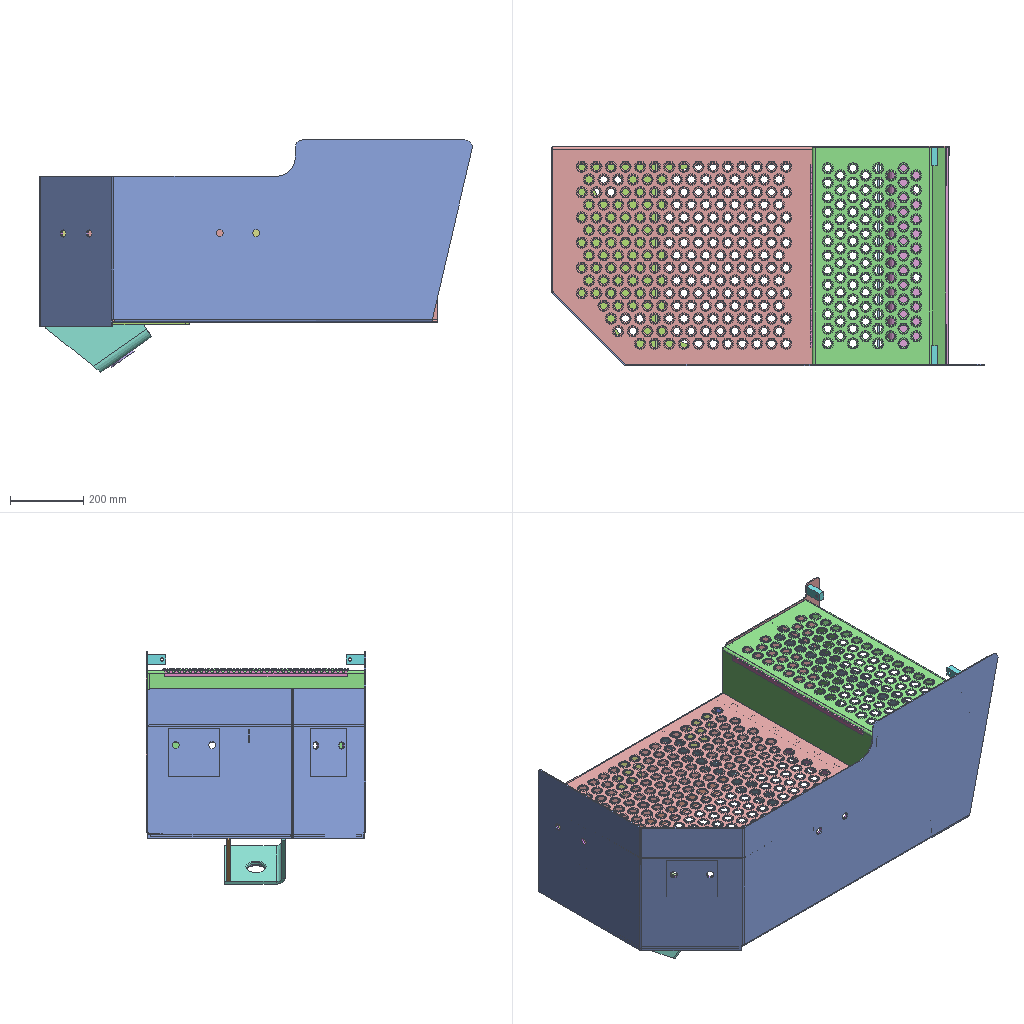Assembly | SolidWorks | 19 different items | 26 placed | box 1185 x 600 x 636 mm
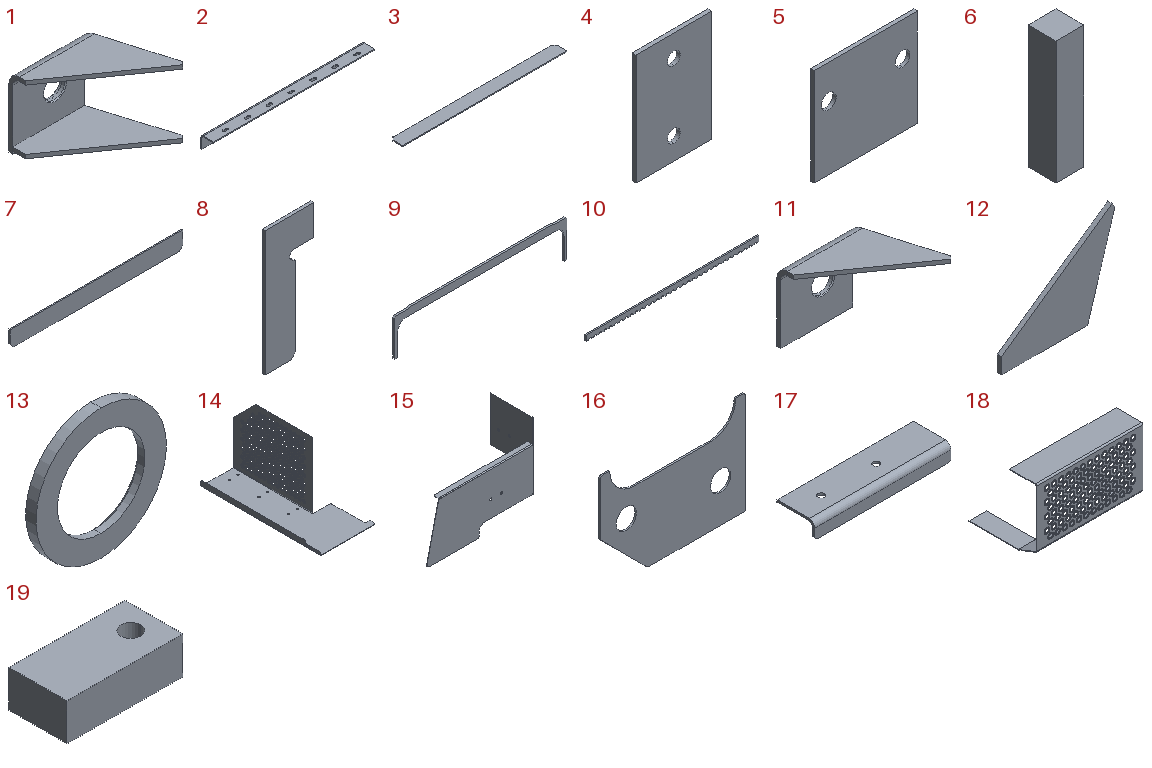Parts list (item | name | quantity | parent item | size | volume | features):
1 | (subassembly) | x1 | - | 224.289 x 199.117 x 166 mm | 593730 mm3 | features CosmeticWeldCutList 1
2 | - | x1 | - | 589 x 47 x 45 mm | 158032 mm3 | features FlatPattern 1, ICE 1, SMBaseFlange 1, SheetMetal 1
3 | - | x2 | - | 593.5 x 45 x 3.2 mm | 85144 mm3 | features Chamfer 1, FlatPattern 1, SMBaseFlange 1, SheetMetal 1
4 | - | x3 | - | 90 x 4.5 x 132 mm | 51870 mm3 | features FlatPattern 1, SMBaseFlange 1, SheetMetal 1
5 | - | x3 | - | 140 x 4.5 x 132 mm | 80333 mm3 | features FlatPattern 1, SMBaseFlange 1, SheetMetal 1
6 | - | x2 | - | 9 x 9 x 40 mm | 3240 mm3 | features FlatPattern 1, SMBaseFlange 1, SheetMetal 1
7 | - | x1 | - | 466 x 3.2 x 45 mm | 66784 mm3 | features FlatPattern 1, SMBaseFlange 1, SheetMetal 1
8 | - | x1 | - | 80 x 4.5 x 206 mm | 52392 mm3 | features FlatPattern 1, SMBaseFlange 1, SheetMetal 1
9 | - | x1 | - | 593.5 x 6 x 130 mm | 101926 mm3 | features FlatPattern 1, SMBaseFlange 1, SheetMetal 1
10 | - | x1 | - | 500 x 4.5 x 16 mm | 32268 mm3 | features FlatPattern 1, ICE 1, SMBaseFlange 1, SheetMetal 1
11 | - | x1 | in 1 | 224.289 x 193.117 x 166 mm | 401605 mm3 | features ICE 2, Chamfer 1, FlatPattern 1, SMBaseFlange 1, SheetMetal 1
12 | - | x1 | in 1 | 224.107 x 9 x 184.117 mm | 177492 mm3 | features FlatPattern 1, SMBaseFlange 1, SheetMetal 1
13 | - | x1 | in 1 | 76 x 6 x 76 mm | 14633 mm3 | features Chamfer 1, FlatPattern 1, SMBaseFlange 1, SheetMetal 1
14 | - | x1 | - | 500 x 1087 x 597 mm | 2492497 mm3 | features Fillet 2, FormToolInstance 2, ICE 2, Chamfer 1, EdgeFlange 1, FlatPattern 1, SMBaseFlange 1, SheetMetal 1
15 | - | x1 | - | 1185 x 596.999 x 511 mm | 2337073 mm3 | features SM3dBend 3, FlatPattern 1, SMBaseFlange 1, SheetMetal 1
16 | - | x1 | - | 576 x 6 x 406 mm | 961136 mm3 | features FlatPattern 1, SMBaseFlange 1, SheetMetal 1
17 | - | x1 | - | 593.5 x 165 x 69.5 mm | 1145527 mm3 | features Chamfer 1, FlatPattern 1, ICE 1, SMBaseFlange 1, SheetMetal 1
18 | - | x1 | - | 593.5 x 380.4 x 367 mm | 1180890 mm3 | features FormToolInstance 2, FlatPattern 1, ICE 1, SMBaseFlange 1, SheetMetal 1
19 | - | x2 | - | 50 x 25 x 16 mm | 19092 mm3 | features FlatPattern 1, HoleWzd 1, SMBaseFlange 1, SheetMetal 1
Mates (type | each side: item.copy, entity, surface, feature):
In the top assembly
Coincident | 14.1 face plane Edge-Flange1 | 15.1 face plane Base-Flange1 | 2 times
DistanceDim | 14.1 face plane Edge-Flange1 | 15.1 face plane Base-Flange1
Coincident | 15.1 face plane Base-Flange1 | 16.1 face plane Base-Flange1 | 3 times
Coincident | 15.1 face plane Base-Flange1 | 17.1 face plane Base-Flange1
DistanceDim | 15.1 face plane Base-Flange1 | 17.1 face plane Base-Flange1
DistanceDim | 15.1 face plane Base-Flange1 | 17.1 face cylinder Cut-Extrude1
Coincident | 16.1 face plane Base-Flange1 | 11.1 face plane Cut-Extrude1
DistanceDim | 14.1 face plane Base-Flange1 | 12.1 face plane Base-Flange1
DistanceDim | 11.1 edge | 15.1 face plane Base-Flange1
Coincident | 14.1 face plane Base-Flange1 | 18.1 face plane Base-Flange1
DistanceDim | 18.1 face plane Base-Flange1 | 15.1 face plane Base-Flange1
Coincident | 14.1 face plane Edge-Flange1 | 18.1 face plane Base-Flange1
Coincident | 14.1 face plane Edge-Flange1 | 2.1 face plane Base-Flange1
DistanceDim | 2.1 face plane Base-Flange1 | 15.1 face plane Base-Flange1
DistanceDim | 14.1 face plane Base-Flange1 | 2.1 face plane Base-Flange1
Coincident | 14.1 face plane Edge-Flange1 | 3.1 face plane Base-Flange1
Coincident | 14.1 face plane Base-Flange1 | 3.1 face plane Base-Flange1
DistanceDim | 15.1 face plane Base-Flange1 | 3.1 face plane Base-Flange1
Coincident | 14.1 face plane Edge-Flange1 | 7.1 face plane Base-Flange1
Coincident | 15.1 face plane Base-Flange1 | 7.1 face plane Base-Flange1
DistanceDim | 14.1 face plane Base-Flange1 | 7.1 face plane Base-Flange1
Coincident | 14.1 face plane Base-Flange1 | 8.1 face plane Base-Flange1
Coincident | 18.1 face plane Base-Flange1 | 8.1 face plane Base-Flange1 | 2 times
Coincident | 16.1 face plane Base-Flange1 | 9.1 face plane Base-Flange1
Coincident | 14.1 face plane Base-Flange1 | 9.1 face plane Base-Flange1
DistanceDim | 15.1 face plane Base-Flange1 | 9.1 face plane Base-Flange1
Coincident | 18.1 face plane Base-Flange1 | 3.2 face plane Base-Flange1
Coincident | 14.1 face plane Base-Flange1 | 3.2 face plane Base-Flange1
DistanceDim | 15.1 face plane Base-Flange1 | 3.2 face plane Base-Flange1
Coincident | 14.1 face plane Base-Flange1 | 4.1 face plane Base-Flange1
Concentric | 14.1 face cylinder Cut-Extrude1 | 4.1 face cylinder Base-Flange1 | 2 times
Coincident | 15.1 face plane Base-Flange1 | 5.1 face plane Base-Flange1
Concentric | 15.1 face cylinder Base-Flange1 | 5.1 face cylinder Base-Flange1 | 2 times
Coincident | 15.1 face plane Base-Flange1 | 5.2 face plane Base-Flange1
Concentric | 15.1 face cylinder Base-Flange1 | 5.2 face cylinder Base-Flange1 | 2 times
Coincident | 15.1 face plane Base-Flange1 | 5.3 face plane Base-Flange1
Concentric | 15.1 face cylinder Base-Flange1 | 5.3 face cylinder Base-Flange1 | 2 times
Coincident | 18.1 face plane Base-Flange1 | 10.1 face plane Base-Flange1
DistanceDim | 14.1 face plane Base-Flange1 | 10.1 face plane Base-Flange1
DistanceDim | 10.1 face plane Base-Flange1 | 18.1 face plane Base-Flange1
Coincident | 17.1 face plane Base-Flange1 | 6.1 face plane Base-Flange1
DistanceDim | 6.1 face plane Base-Flange1 | 14.1 face plane Base-Flange1
DistanceDim | 17.1 face cylinder Cut-Extrude1 | 6.1 face plane Base-Flange1
Coincident | 15.1 face plane Base-Flange1 | 19.1 face plane Base-Flange1
DistanceDim | 14.1 face plane Base-Flange1 | 19.1 face plane Base-Flange1
DistanceDim | 18.1 face plane Base-Flange1 | 19.1 face cylinder M10 Tapped Hole1
Coincident | 14.1 face plane Base-Flange1 | 19.2 face plane Base-Flange1
Coincident | 19.1 face plane Base-Flange1 | 19.2 face plane Base-Flange1 | 2 times
In subassembly 1
Coincident | 11.2 face plane Base-Flange1 | 12.2 face plane Base-Flange1 | 2 times
DistanceDim | 12.2 face plane Base-Flange1 | 11.2 face plane Base-Flange1
Coincident | 11.2 face plane Base-Flange1 | 13.1 face plane Base-Flange1
Concentric | 11.2 face cylinder Cut-Extrude2 | 13.1 face cylinder Base-Flange1
Parallel | 13.1 plane | 1.1 plane